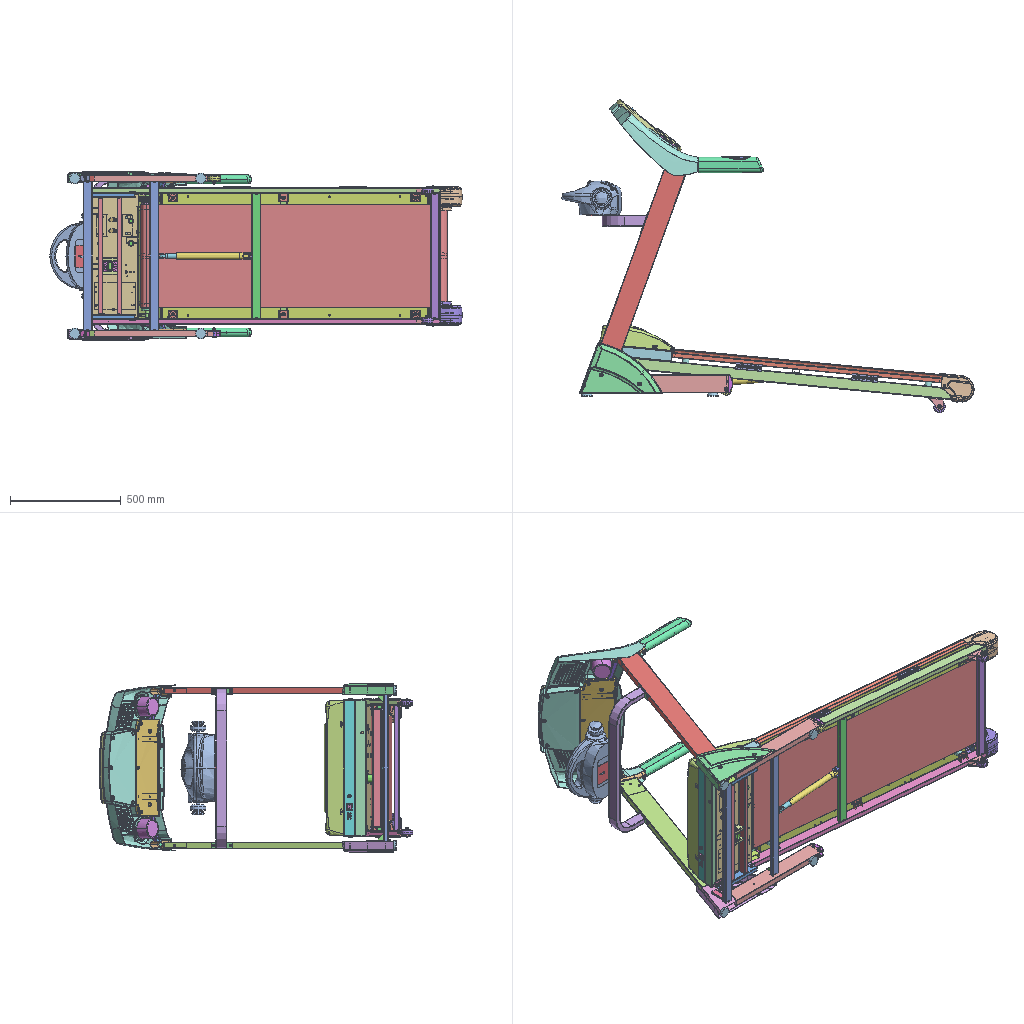Assembly | STEP file | 112 different items | 225 placed | box 1860 x 1415 x 761 mm
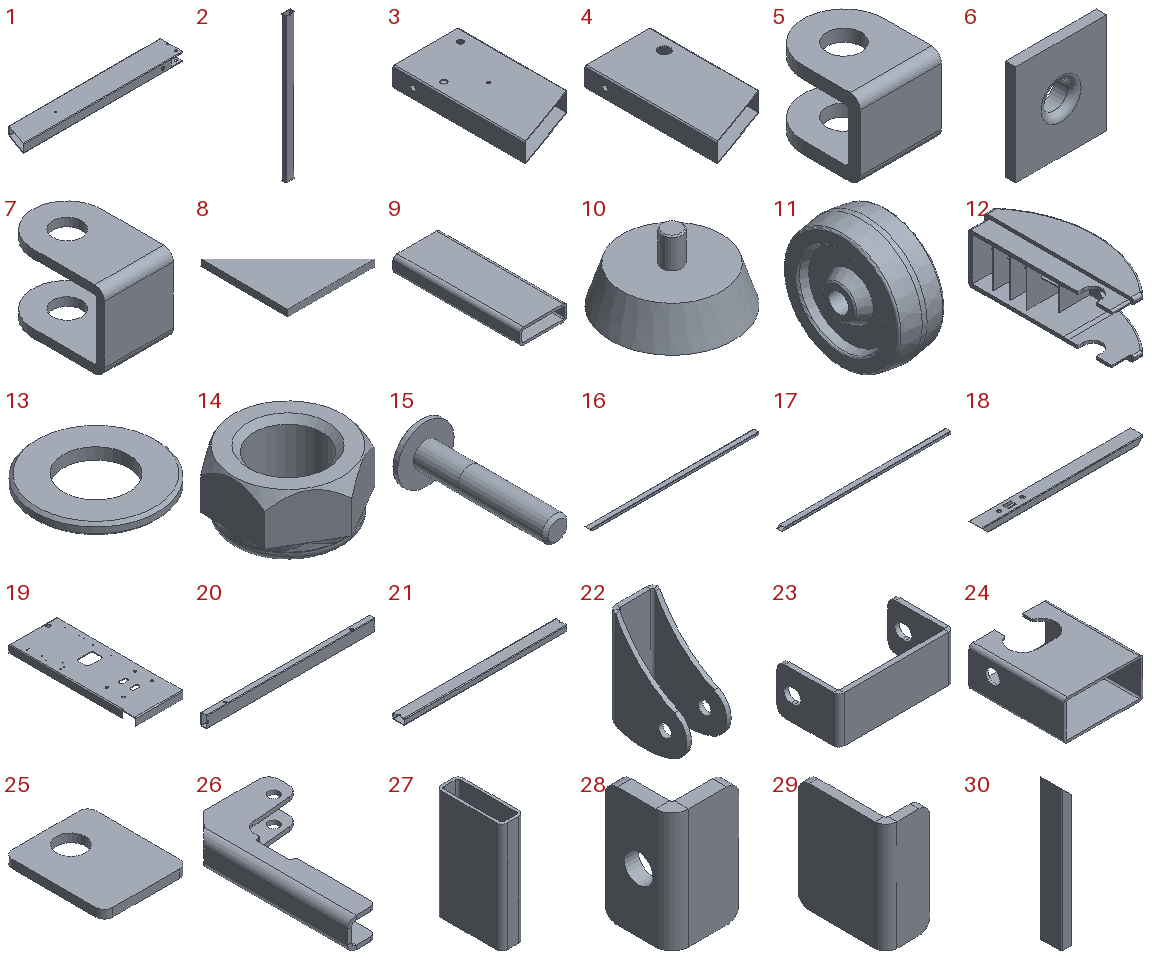Parts list (item | name | quantity | parent item | size | volume):
1 | 7470101 | x2 | in 7470100 | 550 x 80 x 30 mm | 167910 mm3
2 | 7470102 | x2 | in 7470100 | 40 x 20 x 670 mm | 111433 mm3
3 | 7470103L | x1 | in 7470100 | 100 x 200 x 30 mm | 68376 mm3
4 | 7470103R | x1 | in 7470100 | 100 x 200 x 30 mm | 68036 mm3
5 | PN_0004 default | x1 | in 7470100 | 20 x 24 x 19 mm | 3011 mm3
6 | 7470105 | x2 | in 7470100 | 27 x 6 x 30 mm | 2422 mm3
7 | 7470106 | x4 | in 7470100, 7470500 | 25 x 38.5 x 28 mm | 6374 mm3
8 | 7470107 | x4 | in 7470100 | 40 x 40 x 3 mm | 2400 mm3
9 | 7470109 | x2 | in 7470100 | 30 x 80 x 10 mm | 8519 mm3
10 | 7470103W | x4 | in 7470100Z | 48.954 x 48.954 x 27.5 mm | 24706 mm3
11 | PN_0006 default | x1 | in 7470100Z | 22 x 52.843 x 52.843 mm | 34026 mm3
12 | 7470102W | x2 | in 7470100Z | 30 x 80 x 30 mm | 16145 mm3
13 | PN_0021 default | x7 | in 7470100Z, 7470500Z | 17 x 17 x 1.6 mm | 252.969 mm3
14 | N208078 | x4 | in 7470100Z, 7470500Z | 13.017 x 15.011 x 7.5 mm | 666.866 mm3
15 | PN_0023 default | x4 | in 7470100Z, 7470500Z | 18 x 46.451 x 18 mm | 2805 mm3
16 | 7470501L | x1 | in 7470500 | 1650 x 50 x 25 mm | 346400 mm3
17 | 7470501R | x1 | in 7470500 | 1650 x 50 x 25 mm | 346388 mm3
18 | 7470502 | x1 | in 7470500 | 613 x 50 x 25 mm | 116984 mm3
19 | PN_0005 default | x1 | in 7470500 | 210 x 564 x 33 mm | 419212 mm3
20 | 7470504 | x1 | in 7470500 | 565 x 20 x 40 mm | 94145 mm3
21 | 7470505 | x1 | in 7470500 | 565 x 40 x 20 mm | 93951 mm3
22 | 7470506 | x2 | in 7470500 | 30 x 53 x 70.522 mm | 17329 mm3
23 | 7470507 | x2 | in 7470500 | 75 x 40 x 30 mm | 12701 mm3
24 | 7470508 | x1 | in 7470500 | 50 x 60 x 25 mm | 11554 mm3
25 | 7470509 | x1 | in 7470500 | 50 x 60 x 5 mm | 13731 mm3
26 | 7470510 | x1 | in 7470500 | 84 x 160 x 29 mm | 53248 mm3
27 | 7470511 | x2 | in 7470500 | 10 x 30 x 50 mm | 4316 mm3
28 | 7470513 | x4 | in 7470500 | 14 x 14 x 25 mm | 1710 mm3
29 | 7470514 | x2 | in 7470500 | 10 x 20 x 25 mm | 1357 mm3
30 | 7470515 | x1 | in 7470500 | 25 x 50 x 325 mm | 66092 mm3
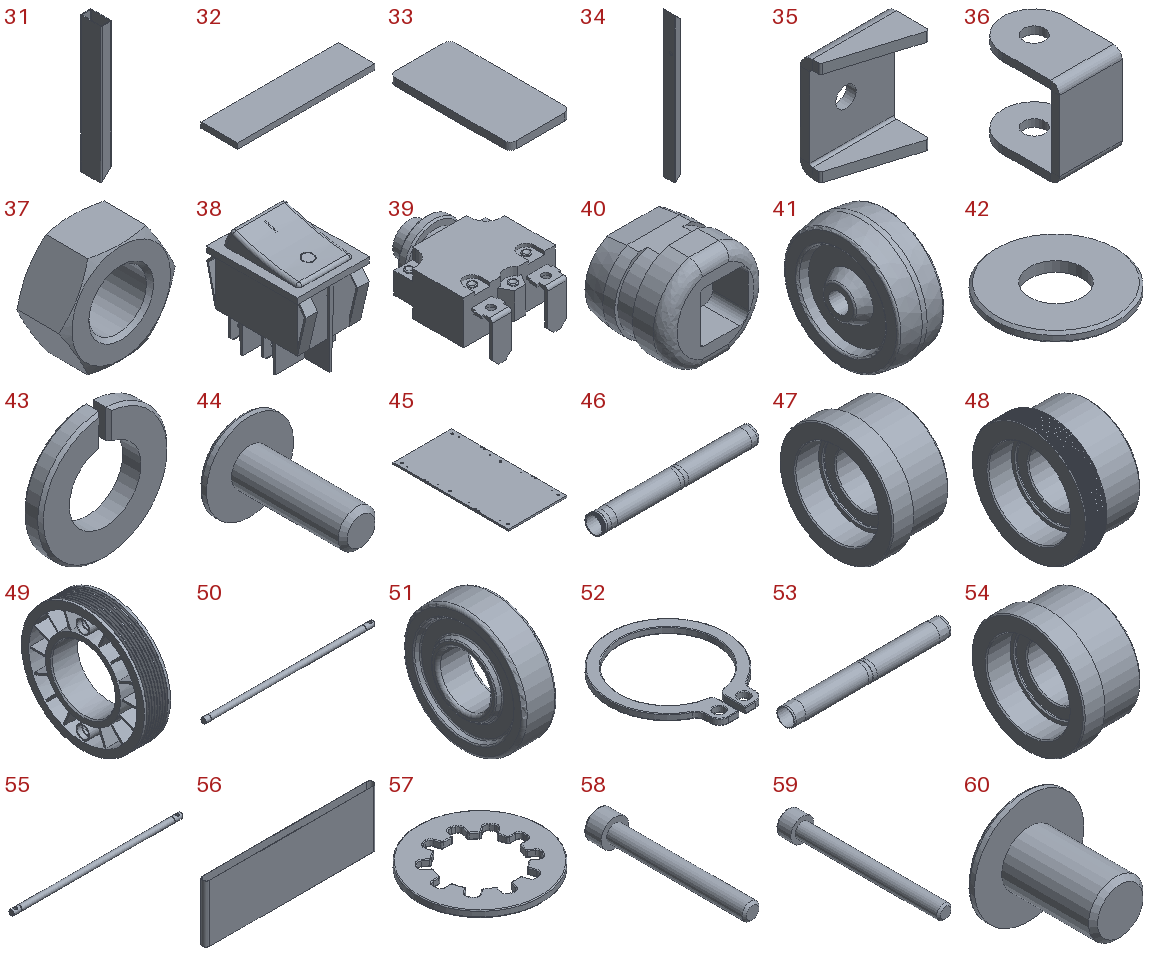31 | 7470516 | x1 | in 7470500 | 25 x 50 x 325 mm | 65710 mm3
32 | 7470517 | x2 | in 7470500 | 75 x 20 x 3 mm | 4500 mm3
33 | 7470518 | x2 | in 7470500 | 25 x 50 x 3 mm | 3734 mm3
34 | 7470519 | x1 | in 7470500 | 25 x 50 x 613 mm | 123960 mm3
35 | 7470520 | x6 | in 7470500 | 35 x 18.649 x 43 mm | 8130 mm3
36 | 7470521 | x1 | in 7470500 | 25 x 35 x 35 mm | 6553 mm3
37 | N108078 | x13 | in 7470500, 7470201LZ, 7470201RZ | 16.166 x 7 x 14 mm | 821.972 mm3
38 | EP002 | x1 | in 7470500Z | 25 x 34.5 x 34.784 mm | 14567 mm3
39 | EC002 | x1 | in 7470500Z | 29.3 x 39.3 x 19.65 mm | 10331 mm3
40 | SB6R-3_Default | x1 | in 7470500Z | 17 x 14 x 16 mm | 1519 mm3
41 | PN_0003 default | x2 | in 7470500Z | 22 x 52.843 x 52.843 mm | 34026 mm3
42 | PN_0020 default | x6 | in 7470500Z | 9.8 x 9.8 x 0.8 mm | 48.045 mm3
43 | W204009 | x5 | in 7470500Z | 9.2 x 1.3 x 9.193 mm | 57.255 mm3
44 | SD10412 | x8 | in 7470500Z | 9.4 x 14.503 x 9.4 mm | 245.335 mm3
45 | DECAK 601 | x1 | in 7470500Z | 605 x 1200 x 18 mm | 13037352 mm3
46 | PN_0001 default | x1 | in 7470700ZA | 495 x 56 x 56 mm | 244128 mm3
47 | PN_0008 default | x1 | in 7470700ZA | 30 x 55.001 x 55.001 mm | 38129 mm3
48 | PN_0011 default | x1 | in 7470700ZA | 30 x 55.999 x 56 mm | 38879 mm3
49 | PN_0010 default | x1 | in 7470700ZA | 23 x 108.001 x 108.001 mm | 96628 mm3
50 | 7470702 | x1 | in 7470700Z | 565 x 17 x 17 mm | 128589 mm3
51 | PL6203ZZA default | x4 | in 7470700Z, 7470800Z | 11 x 40 x 40 mm | 9892 mm3
52 | PN_0012 default | x4 | in 7470700Z, 7470800Z | 19 x 21.5 x 1 mm | 101.865 mm3
53 | PN_0009 default | x1 | in 7470800ZA | 485 x 56 x 56 mm | 236794 mm3
54 | PN_0002 default | x2 | in 7470800ZA | 30 x 54.43 x 54.43 mm | 37639 mm3
55 | 7470803 | x1 | in 7470800Z | 560 x 17 x 17 mm | 125657 mm3
56 | RUBE 601 | x1 | in 7470500Z | 1389 x 59.2 x 465 mm | 2113671 mm3
57 | PN_0018 default | x3 | in 7470500Z | 15 x 15 x 0.8 mm | 82.689 mm3
58 | SA10865 | x1 | in 7470500Z | 13 x 73 x 13 mm | 4160 mm3
59 | SA10880 | x2 | in 7470500Z | 13 x 88 x 13 mm | 4914 mm3
60 | SD10610 | x3 | in 7470500Z | 12 x 12.964 x 12 mm | 479.053 mm3
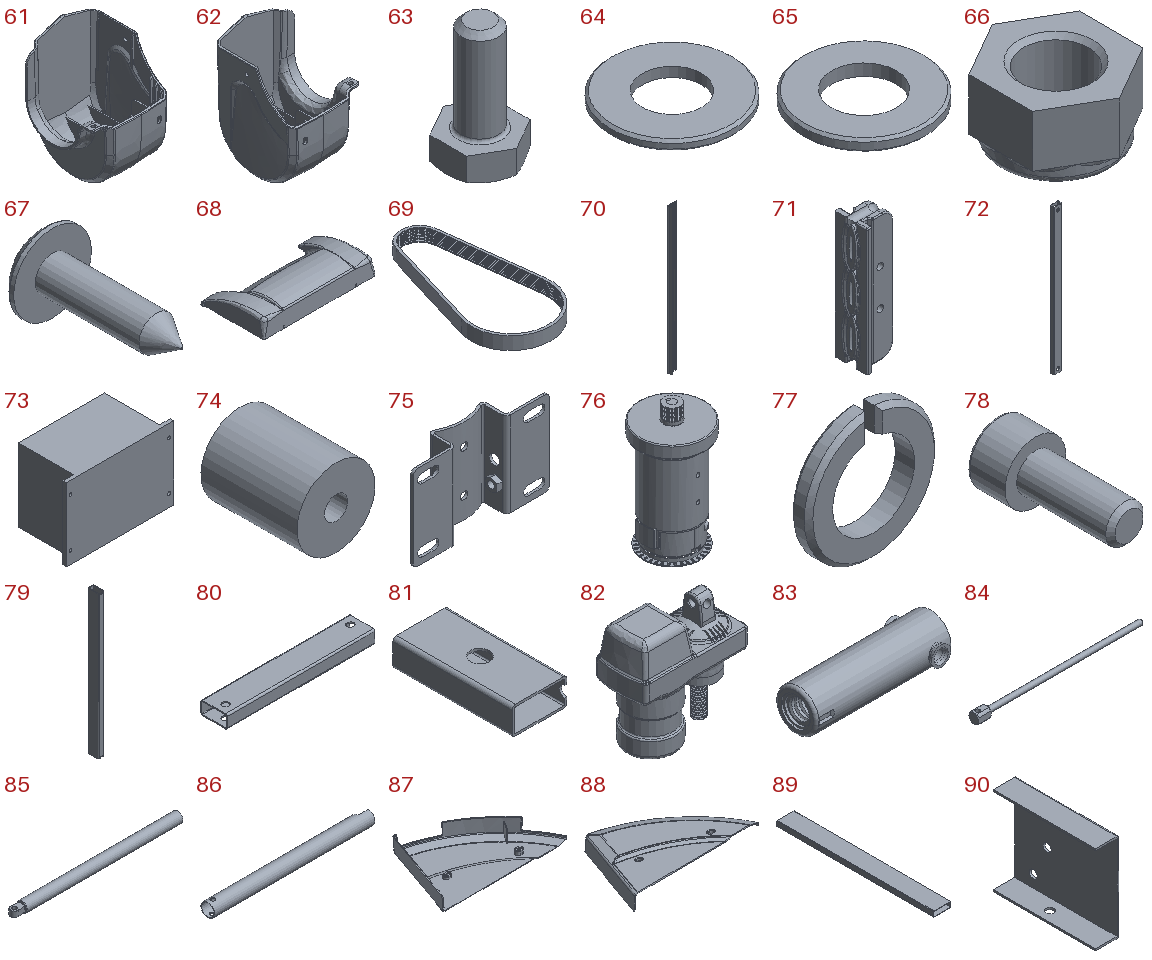61 | EDN CAP 601L | x1 | in 7470500Z | - | 183620 mm3
62 | EDN CAP 601R | x1 | in 7470500Z | - | 183322 mm3
63 | SI1025_M10 | x4 | in 7470500Z | 17 x 19.6 x 32 mm | 3678 mm3
64 | PN_0019 default | x4 | in 7470500Z | 25 x 25 x 2 mm | 736.18 mm3
65 | PN_0022 default | x4 | in 7470500Z | 21 x 21 x 2 mm | 492.233 mm3
66 | N210095 | x4 | in 7470500Z | 17 x 19.63 x 10.5 mm | 1722 mm3
67 | SD20415 | x2 | in 7470500Z | 9 x 17.646 x 9 mm | 255.973 mm3
68 | 96L | x1 | in 7470500Z | - | -
69 | DE200JS8 | x1 | in 7470500Z | 111 x 221.3 x 18 mm | 22925 mm3
70 | SIDE | x2 | in 7470500Z | 76 x 36.5 x 1228 mm | 489204 mm3
71 | jianzhendian | x2 | in 7470500Z | 30 x 30 x 117 mm | 56101 mm3
72 | 7470901 | x1 | in 7470500Z | 30 x 15 x 555 mm | 54621 mm3
73 | Inverter | x1 | in 7470500Z | 185 x 101 x 126 mm | 1922919 mm3
74 | DECH02 | x4 | in 7470500Z | 30 x 37 x 30 mm | 23800 mm3
75 | 6100601 | x1 | in 6100600Z | 160 x 30 x 100 mm | 59957 mm3
76 | MOTOR 602 | x1 | in 6100600Z | - | -
77 | W208016 | x2 | in 6100600Z | 13.5 x 2 x 13.481 mm | 158.687 mm3
78 | SA10820 | x2 | in 6100600Z | 13 x 28 x 13 mm | 1898 mm3
79 | PN_0007 default | x2 | in 7470400 | 20 x 40 x 532 mm | 88457 mm3
80 | 7470402 | x2 | in 7470400 | 225 x 40 x 20 mm | 36971 mm3
81 | 7470403 | x2 | in 7470400 | 30 x 65 x 15 mm | 6216 mm3
82 | PN_0016 default | x1 | in 747 | 148.1 x 70.5 x 151.812 mm | 777031 mm3
83 | J09 601B | x1 | in 747 | 115 x 41.999 x 35 mm | 49295 mm3
84 | GAS SHOCK 609S | x1 | in 747 | 353.5 x 20 x 20 mm | 34694 mm3
85 | GAS SHOCK 609X | x1 | in 747 | 359 x 22 x 22 mm | 94119 mm3
86 | GAS SHOCK 610W | x1 | in 747 | 330 x 28 x 28 mm | 39789 mm3
87 | Right column cover | x1 | in 747 | 372.789 x 229.022 x 48 mm | 179177 mm3
88 | Left column cover | x1 | in 747 | 372.789 x 229.022 x 48 mm | 179176 mm3
89 | 7470201L | x1 | in 7470201LZ | 100 x 900 x 30 mm | 338694 mm3
90 | 7470108L | x2 | in 7470201LZ, 7471200 | 25 x 110 x 95 mm | 30377 mm3
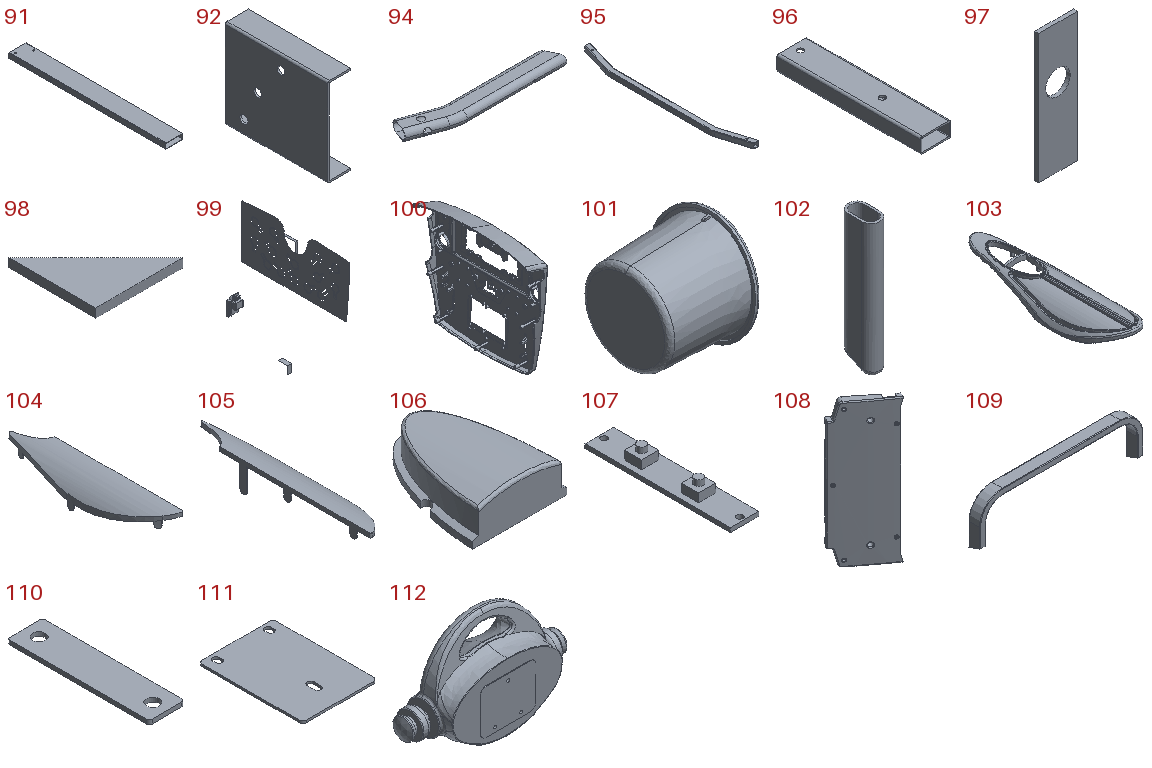91 | 7470201R | x1 | in 7470201RZ | 100 x 900 x 30 mm | 338694 mm3
92 | 7470108R | x2 | in 7470201RZ, 7471200 | 25 x 110 x 95 mm | 30377 mm3
93 | 2_1_9_1 | x1 | in 7471200Z | - | -
94 | 7471201 | x2 | in 7471200 | 428.432 x 98.424 x 30 mm | 88496 mm3
95 | 7471202 | x1 | in 7471200 | 59.901 x 660.964 x 20 mm | 72312 mm3
96 | 7471203 | x2 | in 7471200 | 30 x 140 x 15 mm | 17020 mm3
97 | 7471205 | x2 | in 7471200 | 30 x 3 x 100 mm | 8149 mm3
98 | 7471206 | x2 | in 7471200 | 30 x 30 x 3 mm | 1350 mm3
99 | _3_1_258_20 | x1 | in 7471200Z | - | -
100 | MANIFOLD_SOLID_BREP_204099 | x1 | in 7471200Z | 84.491 x 387.927 x 387.413 mm | 502411 mm3
101 | MANIFOLD_SOLID_BREP_178783_1_1 | x2 | in 7471200Z | 85.183 x 102 x 102 mm | 73233 mm3
102 | Part 6 | x2 | in 7471200Z | 40 x 70 x 294.303 mm | 238300 mm3
103 | - | x1 | - | 40 x 127.347 x 22.5 mm | 10331 mm3
104 | - | x1 | - | 15.6 x 84.944 x 14.464 mm | 720.197 mm3
105 | - | x1 | - | 15.6 x 84.944 x 14.464 mm | 720.173 mm3
106 | - | x1 | - | 16.389 x 20.4 x 8.5 mm | 856.443 mm3
107 | - | x1 | - | 10 x 51 x 6.5 mm | 997.87 mm3
108 | HG_1_1_1 | x1 | in 7471200Z | 138.811 x 117.873 x 440 mm | 209131 mm3
109 | 7471301 | x1 | in 7471300 | 720 x 50 x 200 mm | 206564 mm3
110 | 7471302 | x2 | in 7471300 | 25 x 100 x 3 mm | 7108 mm3
111 | 7471303 | x1 | in 7471300 | 100 x 140 x 3 mm | 40958 mm3
112 | M11404W | x1 | in 747 | 430 x 154.443 x 270 mm | 5728271 mm3
Placements (level | parent | child | x y z in mm | rotation matrix by rows):
1 | 747 | 7470100Z | 319.734 -99.186 350.0 | 1 0 0 0 1 0 0 0 1
2 | 7470100Z | 7470100 | -0.0 -0.0 -0.0 | 1 0 0 0 1 0 0 0 1
3 | 7470100 | 7470101 | -0.0 -0.0 -0.0 | 1 0 0 0 1 0 0 0 1
3 | 7470100 | 7470101 | -0.0 -0.0 -700.0 | 1 0 0 0 1 0 0 0 1
3 | 7470100 | 7470102 | -280.0 20.0 -350.0 | 1 0 0 0 1 0 0 0 1
3 | 7470100 | 7470102 | -580.0 20.0 -350.0 | 1 0 0 0 1 0 0 0 1
3 | 7470100 | 7470103L | -609.433 -17.101 -0.0 | 0.9397 0.342 0 -0.342 0.9397 0 0 0 1
3 | 7470100 | 7470103R | -609.433 -17.101 -700.0 | 0.9397 0.342 0 -0.342 0.9397 0 0 0 1
3 | 7470100 | PN_0004 default | -260.0 30.0 -350.0 | 0 1 0 -1 0 0 0 0 1
3 | 7470100 | 7470105 | -638.73 0.0 0.0 | 0 0 -1 0 1 0 1 0 -0
3 | 7470100 | 7470105 | -638.73 0.0 -700.0 | 0 0 1 0 1 0 -1 0 0
3 | 7470100 | 7470106 | -580.0 40.0 -74.0 | 1 0 0 0 1 0 0 0 1
3 | 7470100 | 7470106 | -580.0 40.0 -626.0 | 1 0 0 0 1 0 0 0 1
3 | 7470100 | 7470107 | -560.0 80.0 -685.0 | 0 0 -1 0 1 0 1 0 0
3 | 7470100 | 7470107 | -563.0 80.0 -15.0 | 0 0 1 0 1 0 -1 0 0
3 | 7470100 | 7470107 | -281.5 80.0 -15.0 | 0 0 1 0 1 0 -1 0 0
3 | 7470100 | 7470107 | -281.5 40.0 -645.0 | 0 0 1 1 0 0 0 1 -0
3 | 7470100 | 7470109 | -599.674 40.0 -672.775 | 1 0 0 0 1 0 0 0 1
3 | 7470100 | 7470109 | -599.674 40.0 -12.775 | 1 0 0 0 1 0 0 0 1
2 | 7470100Z | 7470103W | -638.73 0.0 -0.0 | 0.9991 -0.04147 0 0 0 1 -0.04147 -0.9991 0
2 | 7470100Z | 7470103W | -70.0 -0.0 0.0 | -0.9344 0.3562 0 0 0 1 0.3562 0.9344 0
2 | 7470100Z | PN_0006 default | -10.0 15.0 -0.0 | 0 0 1 0 1 0 -1 0 0
2 | 7470100Z | 7470102W | -0.0 40.0 -0.0 | 1 0 0 0 1 0 0 0 1
2 | 7470100Z | PN_0021 default | -10.0 15.0 -16.6 | 1 0 0 0 1 0 0 0 1
2 | 7470100Z | PN_0021 default | -10.0 15.0 -683.4 | -0.9237 -0.383 0 -0.383 0.9237 0 0 0 -1
2 | 7470100Z | N208078 | -10.0 15.0 -22.1 | 1 0 0 0 1 0 0 0 1
2 | 7470100Z | N208078 | -10.0 15.0 -677.9 | -0.9237 -0.383 0 -0.383 0.9237 0 0 0 -1
2 | 7470100Z | PN_0023 default | -10.0 15.0 15.0 | 1 0 0 0 0 -1 0 1 0
2 | 7470100Z | PN_0023 default | -10.0 15.0 -715.0 | 1 0 0 0 0 1 0 -1 0
2 | 7470100Z | 7470103W | -638.73 0.0 -700.0 | 0.9991 -0.04147 0 0 0 1 -0.04147 -0.9991 0
2 | 7470100Z | 7470103W | -70.0 -0.0 -700.0 | -0.9344 0.3562 0 0 0 1 0.3562 0.9344 0
2 | 7470100Z | 7470102W | -0.0 40.0 -700.0 | 1 0 0 0 1 0 0 0 1
1 | 747 | 7470500Z | 451.203 43.397 310.459 | 0.9955 0.09508 0 -0.09508 0.9955 0 0 0 1
2 | 7470500Z | 7470500 | -0.0 -0.0 -0.0 | 1 0 0 0 1 0 0 0 1
3 | 7470500 | 7470501L | 112.255 -64.436 -15.459 | 1 0 0 0 1 0 0 0 1
3 | 7470500 | 7470501R | 112.255 -64.436 -605.459 | 1 0 0 0 1 0 0 0 1
3 | 7470500 | 7470502 | -700.245 -14.436 -310.459 | 0 0 -1 0 1 0 1 0 0
3 | 7470500 | PN_0005 default | -687.745 -86.436 -310.459 | -1 0 0 0 0 -1 0 -1 0
3 | 7470500 | 7470504 | 867.255 -79.436 -310.459 | 0 0 1 0 1 0 -1 0 -0
3 | 7470500 | 7470505 | 57.255 -79.436 -310.459 | 0 -1 0 0 0 -1 1 0 0
3 | 7470500 | 7470506 | 825.755 -89.436 -17.959 | 0 0 -1 0 1 0 1 0 0
3 | 7470500 | 7470506 | 825.755 -89.436 -602.959 | 0 0 -1 0 1 0 1 0 0
3 | 7470500 | 7470507 | 899.755 -24.436 -32.959 | 1 0 0 0 0 1 0 -1 0
3 | 7470500 | 7470507 | 899.755 -24.436 -587.959 | 1 0 0 0 0 -1 0 1 -0
3 | 7470500 | 7470508 | -442.745 -39.436 -580.459 | 1 0 0 0 1 0 0 0 1
3 | 7470500 | 7470509 | -442.745 -69.436 -32.959 | 1 0 0 0 1 0 0 0 1
3 | 7470500 | 7470510 | -666.745 73.564 -357.459 | 1 0 0 0 1 0 0 0 1
3 | 7470500 | 7470511 | -505.745 -137.337 -252.977 | 0 0 1 -1 0 0 0 -1 0
3 | 7470500 | 7470511 | -662.745 -25.535 -120.977 | 0 0 -1 1 0 0 0 -1 -0
3 | 7470500 | 7470513 | -465.745 10.564 -614.959 | 0 0 -1 0 1 0 1 0 0
3 | 7470500 | 7470513 | -712.745 10.564 -112.959 | 1 0 0 0 1 0 0 0 1
3 | 7470500 | 7470513 | -465.745 10.564 -5.959 | 0 0 1 0 1 0 -1 0 0
3 | 7470500 | 7470513 | -712.745 10.564 -507.959 | 1 0 0 0 1 0 0 0 1
3 | 7470500 | 7470514 | 849.755 -39.436 -2.959 | 0 0 1 0 1 0 -1 0 -0
3 | 7470500 | 7470514 | 849.755 -39.436 -617.959 | 0 0 -1 0 1 0 1 0 0
3 | 7470500 | 7470515 | -387.745 -14.436 -605.459 | 0 0 -1 0 1 0 1 0 0
3 | 7470500 | 7470516 | -712.745 -14.436 -15.459 | 0 0 1 0 1 0 -1 0 -0
3 | 7470500 | 7470517 | 899.755 -42.436 -37.959 | 1 0 0 0 0 1 0 -1 -0
3 | 7470500 | 7470517 | 899.755 -42.436 -582.959 | 1 0 0 0 0 1 0 -1 0
3 | 7470500 | 7470518 | -384.745 -14.436 -15.459 | 0 0 -1 0 1 0 1 0 0
3 | 7470500 | 7470518 | -387.745 -14.436 -605.459 | 0 0 1 0 1 0 -1 0 -0
3 | 7470500 | 7470519 | -700.245 -64.436 -616.959 | 1 0 0 0 1 0 0 0 1
3 | 7470500 | 7470520 | -322.745 -56.436 -27.959 | 0 0 -1 0 1 0 1 0 0
3 | 7470500 | 7470520 | 777.255 -56.436 -27.959 | 0 0 -1 0 1 0 1 0 0
3 | 7470500 | 7470520 | -322.745 -56.436 -592.959 | 0 0 1 0 1 0 -1 0 -0
3 | 7470500 | 7470520 | 777.255 -56.436 -592.959 | 0 0 1 0 1 0 -1 0 -0
3 | 7470500 | 7470520 | 177.255 -36.436 -592.959 | 0 0 1 0 1 0 -1 0 -0
3 | 7470500 | 7470520 | 177.255 -36.436 -27.959 | 0 0 -1 0 1 0 1 0 -0
3 | 7470500 | 7470521 | 37.255 -81.936 -310.459 | 0 -1 0 1 0 0 0 0 1
3 | 7470500 | 7470106 | -502.745 -89.436 -586.459 | 1 0 0 0 -1 0 0 0 -1
3 | 7470500 | 7470106 | -502.745 -89.436 -34.459 | 1 0 0 0 -1 0 0 0 -1
3 | 7470500 | N108078 | -484.245 -80.436 -203.459 | 0 -1 0 0.866 0 -0.5 0.5 0 0.866
3 | 7470500 | N108078 | -322.745 -63.936 -47.959 | 0.866 0 -0.5 0 1 0 0.5 0 0.866
3 | 7470500 | N108078 | -322.745 -63.936 -572.959 | 0.866 0 -0.5 0 1 0 0.5 0 0.866
3 | 7470500 | N108078 | 177.255 -43.936 -47.959 | 0.866 0 -0.5 0 1 0 0.5 0 0.866
3 | 7470500 | N108078 | 777.255 -63.936 -47.959 | 0.866 0 -0.5 0 1 0 0.5 0 0.866
3 | 7470500 | N108078 | 777.255 -63.936 -572.959 | 0.8429 0 -0.5381 0 1 0 0.5381 0 0.8429
3 | 7470500 | N108078 | 177.255 -43.936 -572.959 | 0.866 0 -0.5 0 1 0 0.5 0 0.866
2 | 7470500Z | EP002 | -712.745 -14.186 -485.709 | 0 0 -1 -1 0 0 0 1 0
2 | 7470500Z | EC002 | -655.465 -21.336 -484.294 | 0 -1 0 0 0 -1 1 0 -0
2 | 7470500Z | SB6R-3_Default | -718.245 -14.524 -437.359 | 0 1 0 -1 0 0 0 0 1
2 | 7470500Z | PN_0003 default | 837.255 -127.436 -16.959 | 0 0.005777 -1 0 1 0.005777 1 0 0
2 | 7470500Z | PN_0003 default | 837.255 -127.436 -601.959 | 0 0.01299 0.9999 0 0.9999 -0.01299 -1 0 0
2 | 7470500Z | PN_0020 default | -497.745 -82.636 -532.459 | 1 0 0 0 0 -1 0 1 -0
2 | 7470500Z | PN_0020 default | -590.745 -84.436 -552.459 | 1 0 0 0 0 1 0 -1 0
2 | 7470500Z | PN_0020 default | -662.745 -86.436 -322.459 | 0.9885 -0.1514 0 0 0 1 -0.1514 -0.9885 0
2 | 7470500Z | PN_0020 default | -532.745 -86.436 -382.459 | 1 0 0 0 0 1 0 -1 0
2 | 7470500Z | PN_0020 default | -667.745 -84.436 -532.459 | 0.8986 -0.4389 0 0 0 1 -0.4389 -0.8986 0
2 | 7470500Z | W204009 | -497.745 -82.636 -532.459 | -0.2314 0 0.9729 0 1 0 -0.9729 0 -0.2314
2 | 7470500Z | W204009 | -662.745 -84.336 -322.459 | 0.9816 0 -0.1911 0 -1 0 -0.1911 0 -0.9816
2 | 7470500Z | W204009 | -532.745 -84.336 -382.459 | 1 0 0 0 -1 0 0 0 -1
2 | 7470500Z | W204009 | -667.745 -82.336 -532.459 | 1 0 0 0 -1 0 0 0 -1
2 | 7470500Z | SD10412 | -532.745 -84.336 -382.459 | -0.8802 0 -0.4746 0 1 0 0.4746 0 -0.8802
2 | 7470500Z | SD10412 | -662.745 -84.336 -322.459 | 0.9884 0 0.152 0 1 0 -0.152 0 0.9884
2 | 7470500Z | SD10412 | -497.745 -81.336 -532.459 | 0.8688 0 -0.4951 0 1 0 0.4951 0 0.8688
2 | 7470500Z | SD10412 | -532.745 -81.336 -352.459 | -0.4579 0 -0.889 0 1 0 0.889 0 -0.4579
2 | 7470500Z | PN_0020 default | -532.745 -83.436 -352.459 | 1 0 0 0 0 1 0 -1 0
2 | 7470500Z | W204009 | -532.745 -81.336 -352.459 | 1 0 0 0 -1 0 0 0 -1
2 | 7470500Z | PN_0021 default | 837.255 -127.436 -34.559 | 1 0 0 0 1 0 0 0 1
2 | 7470500Z | PN_0021 default | 837.255 -127.436 -586.359 | -1 0 0 0 1 0 0 0 -1
2 | 7470500Z | PN_0023 default | 837.255 -127.436 -1.959 | 1 0 0 0 0 -1 0 1 -0
2 | 7470500Z | PN_0023 default | 837.255 -127.436 -618.959 | 1 0 0 0 0 1 0 -1 -0
2 | 7470500Z | N208078 | 837.255 -127.436 -40.059 | 1 0 0 0 1 0 0 0 1
2 | 7470500Z | N208078 | 837.255 -127.436 -580.859 | -0.8858 -0.464 0 -0.464 0.8858 0 0 0 -1
2 | 7470500Z | DECAK 601 | 227.255 -10.436 -310.459 | 0 -1 0 0 0 1 -1 0 0
2 | 7470500Z | 7470700Z | -442.745 -24.436 -299.659 | 0 1 0 0 0 -1 -1 0 -0
3 | 7470700Z | 7470700ZA | 0.0 -0.0 0.0 | 1 0 0 0 1 0 0 0 1
4 | 7470700ZA | PN_0001 default | -0.0 -0.0 -0.0 | 1 0 0 0 1 0 0 0 1
4 | 7470700ZA | PN_0008 default | 257.5 0.0 -0.0 | -1 0 0 0 0.5057 -0.8627 0 -0.8627 -0.5057
4 | 7470700ZA | PN_0011 default | -257.5 0.0 -0.0 | 1 0 0 0 1 0 0 0 1
4 | 7470700ZA | PN_0010 default | -257.5 0.0 -0.0 | 1 0 0 0 1 0 0 0 1
3 | 7470700Z | 7470702 | -1.7 -0.0 0.0 | 1 0 0 0 0 1 0 -1 -0
3 | 7470700Z | PL6203ZZA default | 246.5 8.5 -0.0 | 1 0 0 0 1 0 0 0 1
3 | 7470700Z | PL6203ZZA default | -257.5 8.5 -0.0 | 1 0 0 0 1 0 0 0 1
3 | 7470700Z | PN_0012 default | 257.6 -0.0 -0.0 | 0 0 1 0 1 0 -1 0 -0
3 | 7470700Z | PN_0012 default | -258.6 -0.0 0.0 | 0 0 1 0 1 0 -1 0 -0
2 | 7470500Z | 7470800Z | 887.255 -24.436 -309.459 | 0 0 -1 0 1 0 1 0 0
3 | 7470800Z | 7470800ZA | -0.0 0.0 -0.0 | 1 0 0 0 1 0 0 0 1
4 | 7470800ZA | PN_0009 default | -0.0 -0.0 -0.0 | 1 0 0 0 1 0 0 0 1
4 | 7470800ZA | PN_0002 default | -252.5 -0.0 -0.0 | 1 0 0 0 1 0 0 0 1
4 | 7470800ZA | PN_0002 default | 252.5 0.0 0.0 | -1 0 0 0 0.3818 -0.9242 0 -0.9242 -0.3818
3 | 7470800Z | PL6203ZZA default | -252.5 8.5 -0.0 | 1 0 0 0 1 0 0 0 1
3 | 7470800Z | PL6203ZZA default | 241.5 8.5 -0.0 | 1 0 0 0 1 0 0 0 1
3 | 7470800Z | PN_0012 default | 252.6 0.0 -0.0 | 0 0 1 0 1 0 -1 0 0
3 | 7470800Z | PN_0012 default | -252.8 -0.0 -0.0 | 0 0 -1 0 1 0 1 0 0
3 | 7470800Z | 7470803 | -0.0 0.0 -0.0 | 1 0 0 0 1 0 0 0 1
2 | 7470500Z | RUBE 601 | 805.755 -24.436 -310.459 | 1 0 0 0 1 0 0 0 1
2 | 7470500Z | PN_0018 default | 938.055 -24.436 -41.959 | 0 0 -1 0 1 0 1 0 -0
2 | 7470500Z | PN_0018 default | -468.545 -24.436 -577.959 | 0 0 1 0 1 0 -1 0 0
2 | 7470500Z | PN_0021 default | 939.655 -24.436 -41.959 | 0 0 -1 0 1 0 1 0 -0
2 | 7470500Z | PN_0021 default | -470.145 -24.436 -577.959 | 0 0 1 0 1 0 -1 0 0
2 | 7470500Z | SA10865 | -470.145 -24.436 -577.959 | 0 -1 0 1 0 0 0 0 1
2 | 7470500Z | SA10880 | 939.655 -24.436 -41.959 | 0 1 0 -0.891 0 0.4541 0.4541 0 0.891
2 | 7470500Z | SD10412 | 890.255 -81.436 -97.959 | 0 1 0 -1 0 0 0 0 1
2 | 7470500Z | SD10412 | 890.255 -81.436 -522.959 | 0 1 0 -1 0 0 0 0 1
2 | 7470500Z | SD10610 | -465.745 17.564 -2.959 | 0.9957 0 -0.09225 -0.09225 0 -0.9957 0 1 0
2 | 7470500Z | SD10610 | -715.745 17.564 -112.959 | 0 -1 0 1 0 0 0 0 1
2 | 7470500Z | SD10610 | -465.745 17.564 -617.959 | -0.9199 0 0.3922 -0.3922 0 -0.9199 0 -1 -0
2 | 7470500Z | EDN CAP 601L | 824.255 20.504 -42.468 | 0 0 -1 0 1 0 1 0 0
2 | 7470500Z | EDN CAP 601R | 824.255 20.504 -578.45 | 0 0 -1 0 1 0 1 0 -0
2 | 7470500Z | PN_0018 default | 938.055 -24.436 -576.959 | 0 0 -1 0 1 0 1 0 -0
2 | 7470500Z | PN_0021 default | 939.655 -24.436 -576.959 | 0 0 -1 0 1 0 1 0 -0
2 | 7470500Z | SA10880 | 939.655 -24.436 -576.959 | 0 1 0 -0.891 0 0.4541 0.4541 0 0.891
2 | 7470500Z | SI1025_M10 | -650.245 -96.436 -121.428 | 0.7133 -0.7008 0 0 0 1 -0.7008 -0.7133 -0
2 | 7470500Z | SI1025_M10 | -650.245 -96.436 -253.459 | -0.1244 0.9922 0 0 0 1 0.9922 0.1244 -0
2 | 7470500Z | SI1025_M10 | -510.245 -96.436 -153.459 | 0.87 -0.493 0 0 0 1 -0.493 -0.87 -0
2 | 7470500Z | SI1025_M10 | -510.245 -96.436 -253.459 | 0.4078 -0.9131 0 0 0 1 -0.9131 -0.4078 0
2 | 7470500Z | PN_0019 default | -510.245 -84.436 -253.459 | 1 0 0 0 0 -1 0 1 0
2 | 7470500Z | PN_0019 default | -510.245 -84.436 -153.459 | 1 0 0 0 0 -1 0 1 0
2 | 7470500Z | PN_0019 default | -650.245 -84.436 -253.459 | 1 0 0 0 0 -1 0 1 0
2 | 7470500Z | PN_0019 default | -650.245 -84.436 -121.428 | 1 0 0 0 0 -1 0 1 0
2 | 7470500Z | PN_0022 default | -650.245 -79.436 -121.428 | 1 0 0 0 0 -1 0 1 0
2 | 7470500Z | PN_0022 default | -510.245 -79.436 -253.459 | 1 0 0 0 0 -1 0 1 0
2 | 7470500Z | PN_0022 default | -510.245 -79.436 -153.459 | 1 0 0 0 0 -1 0 1 0
2 | 7470500Z | PN_0022 default | -650.245 -79.436 -253.459 | 0.697 0.7171 0 0 0 -1 -0.7171 0.697 0
2 | 7470500Z | N210095 | -650.245 -71.436 -121.428 | 1 0 0 0 0 -1 0 1 0
2 | 7470500Z | N210095 | -650.245 -71.436 -253.459 | 1 0 0 0 0 -1 0 1 0
2 | 7470500Z | N210095 | -510.245 -71.436 -153.459 | 1 0 0 0 0 -1 0 1 0
2 | 7470500Z | N210095 | -510.245 -71.436 -253.459 | 1 0 0 0 0 -1 0 1 0
2 | 7470500Z | SD10412 | 912.255 -96.742 -15.459 | 0.3726 0 -0.928 0 -1 0 -0.928 0 -0.3726
2 | 7470500Z | SD10412 | 912.255 -96.742 -605.459 | -0.0932 0 -0.9956 0 -1 0 -0.9956 0 0.0932
2 | 7470500Z | SD20415 | 851.255 -29.496 4.041 | 1 0 0 0 0 -1 0 1 -0
2 | 7470500Z | SD20415 | 851.255 -29.496 -624.959 | 1 0 0 0 0 1 0 -1 0
2 | 7470500Z | 96L | -545.552 5.354 -310.459 | 0 1 0 0 0 1 1 0 -0
2 | 7470500Z | DE200JS8 | -147.941 454.58 -53.659 | 0.04941 -0.9988 0 0.9988 0.04941 0 0 0 1
2 | 7470500Z | SIDE | 843.255 17.564 0.0413 | 0 0 1 0 1 0 -1 0 0
2 | 7470500Z | SIDE | -384.745 17.564 -620.959 | 0 0 -1 0 1 0 1 0 -0
2 | 7470500Z | jianzhendian | -94.245 -30.366 -13.959 | 0 0 1 0 1 0 -1 0 -0
2 | 7470500Z | jianzhendian | 431.755 -30.366 -13.959 | 0 0 1 0 1 0 -1 0 -0
2 | 7470500Z | 7470901 | 177.255 -26.936 -311.959 | 1 0 0 0 1 0 0 0 1
2 | 7470500Z | Inverter | -564.657 -86.436 -520.108 | 1 0 0 0 1 0 0 0 1
2 | 7470500Z | DECH02 | -322.745 -56.436 -572.959 | 1 0 0 0 1 0 0 0 1
2 | 7470500Z | DECH02 | 777.255 -56.436 -572.959 | 1 0 0 0 1 0 0 0 1
2 | 7470500Z | DECH02 | -322.745 -56.436 -47.959 | 1 0 0 0 1 0 0 0 1
2 | 7470500Z | DECH02 | 777.255 -56.436 -47.959 | 1 0 0 0 1 0 0 0 1
2 | 7470500Z | 6100600Z | -585.745 -83.436 -172.459 | -1 0 0 0 1 0 0 0 -1
3 | 6100600Z | 6100601 | -0.0 0.0 0.0 | 1 0 0 0 1 0 0 0 1
3 | 6100600Z | MOTOR 602 | -0.0 75.0 2.8 | -1 0 0 0 1 0 0 0 -1
3 | 6100600Z | W208016 | -0.0 15.0 25.0 | 1 0 -1e-06 0 1 0 1e-06 0 1
3 | 6100600Z | W208016 | -0.0 15.0 -25.0 | 1 0 -1e-06 0 1 0 1e-06 0 1
3 | 6100600Z | SA10820 | -0.0 15.0 25.0 | 0.02966 0 -0.9996 0 -1 0 -0.9996 0 -0.02966
3 | 6100600Z | SA10820 | -0.0 15.0 -25.0 | -0.9974 0 -0.07138 0 -1 0 -0.07138 0 0.9974
1 | 747 | 7470400 | -117.753 -28.563 -0.0 | 1 0.002646 0 -0.002646 1 0 0 0 1
2 | 7470400 | PN_0007 default | -0.0 -0.0 -0.0 | 1 0 0 0 1 0 0 0 1
2 | 7470400 | PN_0007 default | -85.0 0.0 -0.0 | 1 0 0 0 1 0 0 0 1
2 | 7470400 | 7470402 | -155.0 -0.0 276.0 | 1 0 0 0 1 0 0 0 1
2 | 7470400 | 7470402 | -155.0 -0.0 -276.0 | 1 0 0 0 1 0 0 0 1
2 | 7470400 | 7470403 | -42.5 5.0 -16.5 | 0 1 0 1 0 0 0 0 -1
2 | 7470400 | 7470403 | -42.5 5.0 -76.5 | 0 -1 0 1 0 0 0 0 1
1 | 747 | PN_0016 default | -159.845 95.549 -46.75 | -1 0 0.003316 0.003316 0 1 0 1 0
1 | 747 | J09 601B | -159.898 79.549 -46.75 | -0.003316 0 -1 -1 0 0.003316 0 1 0
1 | 747 | GAS SHOCK 609S | 438.16 -41.107 0.0 | -0.997 0.07682 0 -0.07682 -0.997 0 0 0 1
1 | 747 | GAS SHOCK 609X | 268.656 -54.167 0.0 | 0.997 -0.07682 0 0.07682 0.997 0 0 0 1
1 | 747 | GAS SHOCK 610W | 468.071 -38.802 0.0 | -0.997 -0.07682 0 -0.07682 0.997 0 0 0 -1
1 | 747 | Right column cover | -312.982 -92.7 -19.5 | 1 0.008727 0 -0.008727 1 0 0 0 1
1 | 747 | Left column cover | -312.314 -92.7 19.5 | 1 0.008727 0 -0.008727 1 0 0 0 1
1 | 747 | 7470201LZ | -103.363 579.261 350.0 | 0.9397 0.342 0 -0.342 0.9397 0 0 0 1
2 | 7470201LZ | 7470201L | 62.793 -517.332 -0.0 | 1 0 0 0 1 0 0 0 1
2 | 7470201LZ | 7470108L | 65.095 -487.332 29.981 | 0 0 1 0 -1 0 1 0 -0
2 | 7470201LZ | N108078 | 95.293 -537.332 8.0 | 1 0 0 0 0 -1 0 1 0
2 | 7470201LZ | N108078 | 20.793 -547.332 -0.5 | 0 -1 0 1 0 0 0 0 1
2 | 7470201LZ | N108078 | 30.293 -577.332 8.0 | 1 0 0 0 0 1 0 -1 -0
1 | 747 | 7470201RZ | -25.303 510.595 -350.0 | 0.9397 0.342 0 -0.342 0.9397 0 0 0 1
2 | 7470201RZ | 7470201R | -34.044 -479.505 -0.0 | 1 0 0 0 1 0 0 0 1
2 | 7470201RZ | 7470108R | -31.742 -449.505 6.981 | 0 0 1 0 -1 0 1 0 0
2 | 7470201RZ | N108078 | -66.544 -539.505 -8.0 | 1 0 0.003777 -0.003777 0 1 0 -1 -0
2 | 7470201RZ | N108078 | -1.544 -499.505 -8.0 | -0.9224 0 -0.3861 -0.3861 0 0.9224 0 1 0
2 | 7470201RZ | N108078 | -76.044 -509.505 0.5 | 0 -1 0 -0.3861 0 0.9224 -0.9224 0 -0.3861
1 | 747 | 7471200Z | 60.303 1126.989 -75.496 | 0.6599 0.001418 0.7513 0.7513 -0.001245 -0.6599 0 1 -0.001887
2 | 7471200Z | 2_1_9_1 | -210.526 76.24 200.295 | 1 0 0 0 1 0 0 0 1
2 | 7471200Z | 7471200 | -3.301 406.675 247.983 | 0.6599 0.7513 0 0.001418 -0.001245 1 0.7513 -0.6599 -0.001887
3 | 7471200 | 7471201 | 30.706 -32.369 0.0544 | 1 0 0 0 1 0 0 0 1
3 | 7471200 | 7471201 | 30.706 -32.369 -690.909 | 1 0 0 0 1 0 0 0 1
3 | 7471200 | 7471202 | -189.081 12.311 -330.455 | 0.7513 0 0.6599 -0.6599 0 0.7513 0 -1 0
3 | 7471200 | 7471203 | -243.659 60.252 -199.946 | 0 -0.7513 -0.6599 0 0.6599 -0.7513 1 0 -0
3 | 7471200 | 7471203 | -243.659 60.252 -459.946 | 0 -0.7513 -0.6599 0 0.6599 -0.7513 1 0 -0
3 | 7471200 | 7471205 | -157.467 -40.161 -680.909 | 0 -0.342 -0.9397 0 -0.9397 0.342 -1 0 -0
3 | 7471200 | 7471205 | -158.493 -42.98 20.054 | 0 0.342 -0.9397 0 0.9397 0.342 1 0 -0
3 | 7471200 | 7470108R | -193.952 -147.134 -686.39 | 0 0.342 0.9397 0 0.9397 -0.342 -1 0 0
3 | 7471200 | 7470108L | -193.952 -147.134 -11.426 | 0 0.342 0.9397 0 0.9397 -0.342 -1 0 0
3 | 7471200 | 7471206 | -171.875 -2.802 7.803 | 0.5313 -0.5313 -0.6599 -0.4667 0.4667 -0.7513 0.7071 0.7071 -0
3 | 7471200 | 7471206 | -173.854 -5.056 -668.658 | 0.5313 -0.5313 0.6599 -0.4667 0.4667 0.7513 -0.7071 -0.7071 -0
2 | 7471200Z | _3_1_258_20 | -212.55 76.1 199.638 | 1 0 0 0 1 0 0 0 1
2 | 7471200Z | MANIFOLD_SOLID_BREP_204099 | -210.525 76.237 200.294 | 1 0 0 0 1 -8e-06 0 8e-06 1
2 | 7471200Z | MANIFOLD_SOLID_BREP_178783_1_1 | -209.737 627.688 203.002 | 1 0 0 0 1 0 0 0 1
2 | 7471200Z | MANIFOLD_SOLID_BREP_178783_1_1 | -210.164 76.318 201.386 | 1 0 0 0 1 0 0 0 1
2 | 7471200Z | Part 6 | 131.066 422.108 448.931 | 0 0.7513 -0.6599 1 -0.001245 -0.001418 -0.001887 -0.6599 -0.7513
2 | 7471200Z | Part 6 | 131.139 -268.854 450.306 | 0 0.7513 -0.6599 1 -0.001245 -0.001418 -0.001887 -0.6599 -0.7513
2 | 7471200Z | subassembly 2 | 55.878 415.884 328.125 | -0.1119 -0.6599 0.7429 -0.9887 -0.001418 -0.1502 0.1002 -0.7513 -0.6523
3 | subassembly 2 | subassembly 3 | -4.701 -25.324 -9.045 | 0.9888 0 -0.149 0 1 0 0.149 0 0.9888
3 | subassembly 2 | subassembly 4 | -4.701 -25.255 -9.045 | 0.9883 0 -0.1522 0 1 0 0.1522 0 0.9883
4 | subassembly 4 | subassembly 5 | 0.0 0.0 0.0 | 1 0 0 0 1 0 0 0 1
4 | subassembly 4 | subassembly 6 | 0.0 0.0 0.0 | 1 0 0 0 1 0 0 0 1
3 | subassembly 2 | subassembly 7 | -4.695 65.417 -9.087 | 0.9888 0 -0.149 0 1 0 0.149 0 0.9888
3 | subassembly 2 | subassembly 8 | -5.818 31.104 -1.628 | 0.9888 0 -0.149 0 1 0 0.149 0 0.9888
2 | 7471200Z | HG_1_1_1 | 10.559 462.54 491.44 | 0.6293 0.7771 0 0 0 1 0.7771 -0.6293 -0
1 | 747 | 7471300 | -148.85 694.255 -9.515 | 0 0 -1 0 1 0 1 0 -0
2 | 7471300 | 7471301 | 7.015 -43.852 100.0 | 1 0 0 0 1 0 0 0 1
2 | 7471300 | 7471302 | -345.699 -5.796 -98.845 | 1 0 0 0 0.9397 0.342 0 -0.342 0.9397
2 | 7471300 | 7471302 | 349.301 -5.796 -98.845 | 1 0 0 0 0.9397 0.342 0 -0.342 0.9397
2 | 7471300 | 7471303 | 7.015 6.148 100.0 | 1 0 0 0 0 1 0 -1 0
1 | 747 | M11404W | -281.169 704.904 -0.0 | 0 0 -1 0 1 0 1 0 0